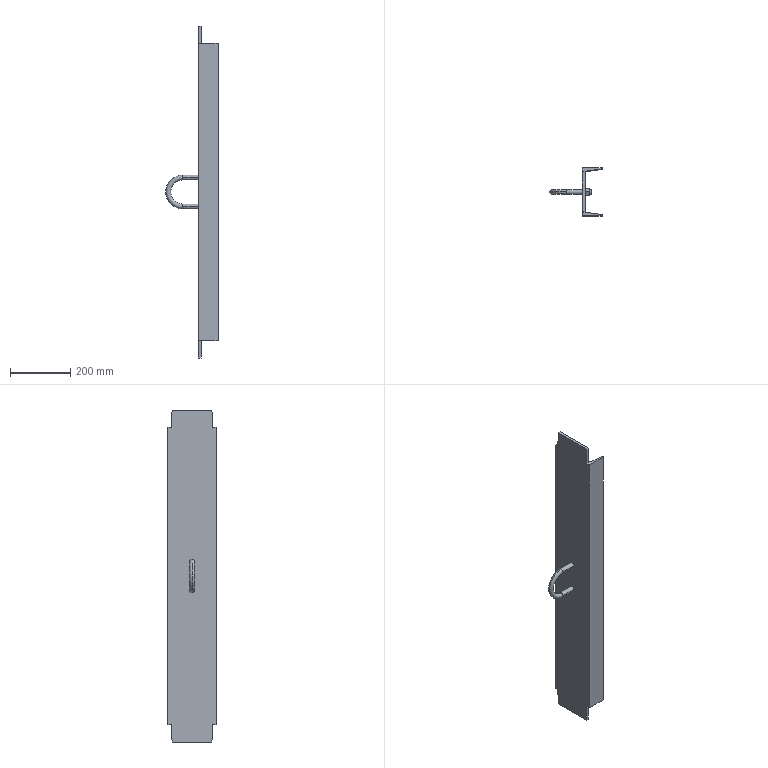Part | SolidWorks | features Extrusion 1, HoleWzd 1, ICE 1, MirrorSolid 1, MoveCopyBody 1, Stock 1, Sweep 1 | 3 solids | 58 faces | box 173 x 160 x 1098 mm | volume 2436946 mm3 | plane 36 | cylinder 12 | cone 8 | torus 2 | commonest cylinder face diameters 16 x8 13.835 x4